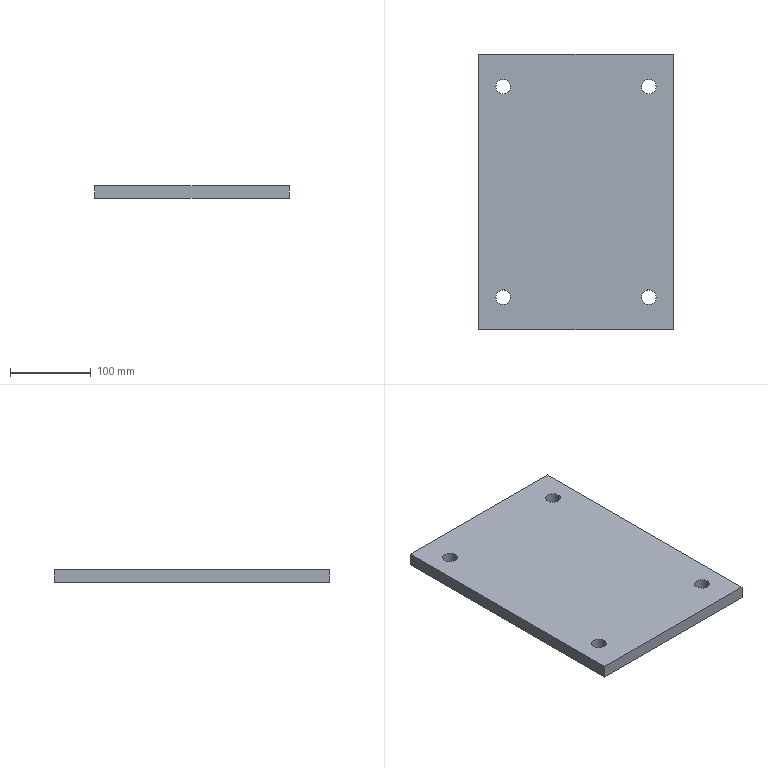Part | SolidWorks | features Extrusion 1 | 1 solid | 14 faces | box 240 x 340 x 16 mm | volume 1289314 mm3 | cylinder 8 | plane 6 | commonest cylinder face diameters 18 x8
STEP:
#1=CARTESIAN_POINT('',(-99.,-130.,16.));
#2=VERTEX_POINT('',#1);
#3=CARTESIAN_POINT('',(-81.,-130.,16.));
#4=VERTEX_POINT('',#3);
#5=CARTESIAN_POINT('',(-90.,-130.,16.));
#6=DIRECTION('',(0.,0.,1.));
#7=DIRECTION('',(1.,0.,0.));
#8=AXIS2_PLACEMENT_3D('',#5,#6,#7);
#9=CIRCLE('',#8,9.);
#10=EDGE_CURVE('',#2,#4,#9,.T.);
#11=ORIENTED_EDGE('',*,*,#10,.T.);
#12=CARTESIAN_POINT('',(-81.,-130.,0.));
#13=VERTEX_POINT('',#12);
#14=CARTESIAN_POINT('',(-81.,-130.,16.));
#15=DIRECTION('',(0.,0.,-1.));
#16=VECTOR('',#15,1000.);
#17=LINE('',#14,#16);
#18=EDGE_CURVE('',#4,#13,#17,.T.);
#19=ORIENTED_EDGE('',*,*,#18,.T.);
#20=CARTESIAN_POINT('',(-99.,-130.,0.));
#21=VERTEX_POINT('',#20);
#22=CARTESIAN_POINT('',(-90.,-130.,0.));
#23=DIRECTION('',(0.,0.,1.));
#24=DIRECTION('',(1.,0.,0.));
#25=AXIS2_PLACEMENT_3D('',#22,#23,#24);
#26=CIRCLE('',#25,9.);
#27=EDGE_CURVE('',#21,#13,#26,.T.);
#28=ORIENTED_EDGE('',*,*,#27,.F.);
#29=CARTESIAN_POINT('',(-99.,-130.,16.));
#30=DIRECTION('',(0.,0.,-1.));
#31=VECTOR('',#30,1000.);
#32=LINE('',#29,#31);
#33=EDGE_CURVE('',#2,#21,#32,.T.);
#34=ORIENTED_EDGE('',*,*,#33,.F.);
#35=EDGE_LOOP('',(#11,#19,#28,#34));
#36=FACE_OUTER_BOUND('',#35,.T.);
#37=CARTESIAN_POINT('',(-90.,-130.,16.));
#38=DIRECTION('',(0.,0.,-1.));
#39=DIRECTION('',(-1.,0.,0.));
#40=AXIS2_PLACEMENT_3D('',#37,#38,#39);
#41=CYLINDRICAL_SURFACE('',#40,9.);
#42=ADVANCED_FACE('',(#36),#41,.F.);
#43=CARTESIAN_POINT('',(81.,-130.,16.));
#44=VERTEX_POINT('',#43);
#45=CARTESIAN_POINT('',(99.,-130.,16.));
#46=VERTEX_POINT('',#45);
#47=CARTESIAN_POINT('',(90.,-130.,16.));
#48=DIRECTION('',(0.,0.,1.));
#49=DIRECTION('',(1.,0.,0.));
#50=AXIS2_PLACEMENT_3D('',#47,#48,#49);
#51=CIRCLE('',#50,9.);
#52=EDGE_CURVE('',#44,#46,#51,.T.);
#53=ORIENTED_EDGE('',*,*,#52,.T.);
#54=CARTESIAN_POINT('',(99.,-130.,0.));
#55=VERTEX_POINT('',#54);
#56=CARTESIAN_POINT('',(99.,-130.,16.));
#57=DIRECTION('',(0.,0.,-1.));
#58=VECTOR('',#57,1000.);
#59=LINE('',#56,#58);
#60=EDGE_CURVE('',#46,#55,#59,.T.);
#61=ORIENTED_EDGE('',*,*,#60,.T.);
#62=CARTESIAN_POINT('',(81.,-130.,0.));
#63=VERTEX_POINT('',#62);
#64=CARTESIAN_POINT('',(90.,-130.,0.));
#65=DIRECTION('',(0.,0.,1.));
#66=DIRECTION('',(1.,0.,0.));
#67=AXIS2_PLACEMENT_3D('',#64,#65,#66);
#68=CIRCLE('',#67,9.);
#69=EDGE_CURVE('',#63,#55,#68,.T.);
#70=ORIENTED_EDGE('',*,*,#69,.F.);
#71=CARTESIAN_POINT('',(81.,-130.,16.));
#72=DIRECTION('',(0.,0.,-1.));
#73=VECTOR('',#72,1000.);
#74=LINE('',#71,#73);
#75=EDGE_CURVE('',#44,#63,#74,.T.);
#76=ORIENTED_EDGE('',*,*,#75,.F.);
#77=EDGE_LOOP('',(#53,#61,#70,#76));
#78=FACE_OUTER_BOUND('',#77,.T.);
#79=CARTESIAN_POINT('',(90.,-130.,16.));
#80=DIRECTION('',(0.,0.,-1.));
#81=DIRECTION('',(-1.,0.,0.));
#82=AXIS2_PLACEMENT_3D('',#79,#80,#81);
#83=CYLINDRICAL_SURFACE('',#82,9.);
#84=ADVANCED_FACE('',(#78),#83,.F.);
#85=CARTESIAN_POINT('',(81.,130.,16.));
#86=VERTEX_POINT('',#85);
#87=CARTESIAN_POINT('',(99.,130.,16.));
#88=VERTEX_POINT('',#87);
#89=CARTESIAN_POINT('',(90.,130.,16.));
#90=DIRECTION('',(0.,0.,1.));
#91=DIRECTION('',(1.,0.,0.));
#92=AXIS2_PLACEMENT_3D('',#89,#90,#91);
#93=CIRCLE('',#92,9.);
#94=EDGE_CURVE('',#86,#88,#93,.T.);
#95=ORIENTED_EDGE('',*,*,#94,.T.);
#96=CARTESIAN_POINT('',(99.,130.,0.));
#97=VERTEX_POINT('',#96);
#98=CARTESIAN_POINT('',(99.,130.,16.));
#99=DIRECTION('',(0.,0.,-1.));
#100=VECTOR('',#99,1000.);
#101=LINE('',#98,#100);
#102=EDGE_CURVE('',#88,#97,#101,.T.);
#103=ORIENTED_EDGE('',*,*,#102,.T.);
#104=CARTESIAN_POINT('',(81.,130.,0.));
#105=VERTEX_POINT('',#104);
#106=CARTESIAN_POINT('',(90.,130.,0.));
#107=DIRECTION('',(0.,0.,1.));
#108=DIRECTION('',(1.,0.,0.));
#109=AXIS2_PLACEMENT_3D('',#106,#107,#108);
#110=CIRCLE('',#109,9.);
#111=EDGE_CURVE('',#105,#97,#110,.T.);
#112=ORIENTED_EDGE('',*,*,#111,.F.);
#113=CARTESIAN_POINT('',(81.,130.,16.));
#114=DIRECTION('',(0.,0.,-1.));
#115=VECTOR('',#114,1000.);
#116=LINE('',#113,#115);
#117=EDGE_CURVE('',#86,#105,#116,.T.);
#118=ORIENTED_EDGE('',*,*,#117,.F.);
#119=EDGE_LOOP('',(#95,#103,#112,#118));
#120=FACE_OUTER_BOUND('',#119,.T.);
#121=CARTESIAN_POINT('',(90.,130.,16.));
#122=DIRECTION('',(0.,0.,-1.));
#123=DIRECTION('',(-1.,0.,0.));
#124=AXIS2_PLACEMENT_3D('',#121,#122,#123);
#125=CYLINDRICAL_SURFACE('',#124,9.);
#126=ADVANCED_FACE('',(#120),#125,.F.);
#127=CARTESIAN_POINT('',(-99.,130.,16.));
#128=VERTEX_POINT('',#127);
#129=CARTESIAN_POINT('',(-81.,130.,16.));
#130=VERTEX_POINT('',#129);
#131=CARTESIAN_POINT('',(-90.,130.,16.));
#132=DIRECTION('',(0.,0.,1.));
#133=DIRECTION('',(1.,0.,0.));
#134=AXIS2_PLACEMENT_3D('',#131,#132,#133);
#135=CIRCLE('',#134,9.);
#136=EDGE_CURVE('',#128,#130,#135,.T.);
#137=ORIENTED_EDGE('',*,*,#136,.T.);
#138=CARTESIAN_POINT('',(-81.,130.,0.));
#139=VERTEX_POINT('',#138);
#140=CARTESIAN_POINT('',(-81.,130.,16.));
#141=DIRECTION('',(0.,0.,-1.));
#142=VECTOR('',#141,1000.);
#143=LINE('',#140,#142);
#144=EDGE_CURVE('',#130,#139,#143,.T.);
#145=ORIENTED_EDGE('',*,*,#144,.T.);
#146=CARTESIAN_POINT('',(-99.,130.,0.));
#147=VERTEX_POINT('',#146);
#148=CARTESIAN_POINT('',(-90.,130.,0.));
#149=DIRECTION('',(0.,0.,1.));
#150=DIRECTION('',(1.,0.,0.));
#151=AXIS2_PLACEMENT_3D('',#148,#149,#150);
#152=CIRCLE('',#151,9.);
#153=EDGE_CURVE('',#147,#139,#152,.T.);
#154=ORIENTED_EDGE('',*,*,#153,.F.);
#155=CARTESIAN_POINT('',(-99.,130.,16.));
#156=DIRECTION('',(0.,0.,-1.));
#157=VECTOR('',#156,1000.);
#158=LINE('',#155,#157);
#159=EDGE_CURVE('',#128,#147,#158,.T.);
#160=ORIENTED_EDGE('',*,*,#159,.F.);
#161=EDGE_LOOP('',(#137,#145,#154,#160));
#162=FACE_OUTER_BOUND('',#161,.T.);
#163=CARTESIAN_POINT('',(-90.,130.,16.));
#164=DIRECTION('',(0.,0.,-1.));
#165=DIRECTION('',(-1.,0.,0.));
#166=AXIS2_PLACEMENT_3D('',#163,#164,#165);
#167=CYLINDRICAL_SURFACE('',#166,9.);
#168=ADVANCED_FACE('',(#162),#167,.F.);
#169=CARTESIAN_POINT('',(120.,-170.,16.));
#170=VERTEX_POINT('',#169);
#171=CARTESIAN_POINT('',(120.,170.,16.));
#172=VERTEX_POINT('',#171);
#173=CARTESIAN_POINT('',(120.,-170.,16.));
#174=DIRECTION('',(0.,1.,0.));
#175=VECTOR('',#174,1000.);
#176=LINE('',#173,#175);
#177=EDGE_CURVE('',#170,#172,#176,.T.);
#178=ORIENTED_EDGE('',*,*,#177,.T.);
#179=CARTESIAN_POINT('',(-120.,170.,16.));
#180=VERTEX_POINT('',#179);
#181=CARTESIAN_POINT('',(-120.,170.,16.));
#182=DIRECTION('',(-1.,0.,0.));
#183=VECTOR('',#182,1000.);
#184=LINE('',#181,#183);
#185=EDGE_CURVE('',#172,#180,#184,.T.);
#186=ORIENTED_EDGE('',*,*,#185,.T.);
#187=CARTESIAN_POINT('',(-120.,-170.,16.));
#188=VERTEX_POINT('',#187);
#189=CARTESIAN_POINT('',(-120.,-170.,16.));
#190=DIRECTION('',(0.,-1.,0.));
#191=VECTOR('',#190,1000.);
#192=LINE('',#189,#191);
#193=EDGE_CURVE('',#180,#188,#192,.T.);
#194=ORIENTED_EDGE('',*,*,#193,.T.);
#195=CARTESIAN_POINT('',(-120.,-170.,16.));
#196=DIRECTION('',(1.,0.,0.));
#197=VECTOR('',#196,1000.);
#198=LINE('',#195,#197);
#199=EDGE_CURVE('',#188,#170,#198,.T.);
#200=ORIENTED_EDGE('',*,*,#199,.T.);
#201=EDGE_LOOP('',(#178,#186,#194,#200));
#202=FACE_OUTER_BOUND('',#201,.T.);
#203=ORIENTED_EDGE('',*,*,#136,.F.);
#204=CARTESIAN_POINT('',(-90.,130.,16.));
#205=DIRECTION('',(0.,0.,1.));
#206=DIRECTION('',(1.,0.,0.));
#207=AXIS2_PLACEMENT_3D('',#204,#205,#206);
#208=CIRCLE('',#207,9.);
#209=EDGE_CURVE('',#130,#128,#208,.T.);
#210=ORIENTED_EDGE('',*,*,#209,.F.);
#211=EDGE_LOOP('',(#203,#210));
#212=FACE_BOUND('',#211,.T.);
#213=ORIENTED_EDGE('',*,*,#94,.F.);
#214=CARTESIAN_POINT('',(90.,130.,16.));
#215=DIRECTION('',(0.,0.,1.));
#216=DIRECTION('',(1.,0.,0.));
#217=AXIS2_PLACEMENT_3D('',#214,#215,#216);
#218=CIRCLE('',#217,9.);
#219=EDGE_CURVE('',#88,#86,#218,.T.);
#220=ORIENTED_EDGE('',*,*,#219,.F.);
#221=EDGE_LOOP('',(#213,#220));
#222=FACE_BOUND('',#221,.T.);
#223=ORIENTED_EDGE('',*,*,#52,.F.);
#224=CARTESIAN_POINT('',(90.,-130.,16.));
#225=DIRECTION('',(0.,0.,1.));
#226=DIRECTION('',(1.,0.,0.));
#227=AXIS2_PLACEMENT_3D('',#224,#225,#226);
#228=CIRCLE('',#227,9.);
#229=EDGE_CURVE('',#46,#44,#228,.T.);
#230=ORIENTED_EDGE('',*,*,#229,.F.);
#231=EDGE_LOOP('',(#223,#230));
#232=FACE_BOUND('',#231,.T.);
#233=ORIENTED_EDGE('',*,*,#10,.F.);
#234=CARTESIAN_POINT('',(-90.,-130.,16.));
#235=DIRECTION('',(0.,0.,1.));
#236=DIRECTION('',(1.,0.,0.));
#237=AXIS2_PLACEMENT_3D('',#234,#235,#236);
#238=CIRCLE('',#237,9.);
#239=EDGE_CURVE('',#4,#2,#238,.T.);
#240=ORIENTED_EDGE('',*,*,#239,.F.);
#241=EDGE_LOOP('',(#233,#240));
#242=FACE_BOUND('',#241,.T.);
#243=CARTESIAN_POINT('',(0.,0.,16.));
#244=DIRECTION('',(0.,0.,-1.));
#245=DIRECTION('',(-1.,0.,0.));
#246=AXIS2_PLACEMENT_3D('',#243,#244,#245);
#247=PLANE('',#246);
#248=ADVANCED_FACE('',(#202,#212,#222,#232,#242),#247,.F.);
#249=ORIENTED_EDGE('',*,*,#69,.T.);
#250=CARTESIAN_POINT('',(90.,-130.,0.));
#251=DIRECTION('',(0.,0.,1.));
#252=DIRECTION('',(1.,0.,0.));
#253=AXIS2_PLACEMENT_3D('',#250,#251,#252);
#254=CIRCLE('',#253,9.);
#255=EDGE_CURVE('',#55,#63,#254,.T.);
#256=ORIENTED_EDGE('',*,*,#255,.T.);
#257=EDGE_LOOP('',(#249,#256));
#258=FACE_BOUND('',#257,.T.);
#259=ORIENTED_EDGE('',*,*,#153,.T.);
#260=CARTESIAN_POINT('',(-90.,130.,0.));
#261=DIRECTION('',(0.,0.,1.));
#262=DIRECTION('',(1.,0.,0.));
#263=AXIS2_PLACEMENT_3D('',#260,#261,#262);
#264=CIRCLE('',#263,9.);
#265=EDGE_CURVE('',#139,#147,#264,.T.);
#266=ORIENTED_EDGE('',*,*,#265,.T.);
#267=EDGE_LOOP('',(#259,#266));
#268=FACE_BOUND('',#267,.T.);
#269=CARTESIAN_POINT('',(120.,-170.,0.));
#270=VERTEX_POINT('',#269);
#271=CARTESIAN_POINT('',(120.,170.,0.));
#272=VERTEX_POINT('',#271);
#273=CARTESIAN_POINT('',(120.,-170.,0.));
#274=DIRECTION('',(0.,1.,0.));
#275=VECTOR('',#274,1000.);
#276=LINE('',#273,#275);
#277=EDGE_CURVE('',#270,#272,#276,.T.);
#278=ORIENTED_EDGE('',*,*,#277,.F.);
#279=CARTESIAN_POINT('',(-120.,-170.,0.));
#280=VERTEX_POINT('',#279);
#281=CARTESIAN_POINT('',(-120.,-170.,0.));
#282=DIRECTION('',(1.,0.,0.));
#283=VECTOR('',#282,1000.);
#284=LINE('',#281,#283);
#285=EDGE_CURVE('',#280,#270,#284,.T.);
#286=ORIENTED_EDGE('',*,*,#285,.F.);
#287=CARTESIAN_POINT('',(-120.,170.,0.));
#288=VERTEX_POINT('',#287);
#289=CARTESIAN_POINT('',(-120.,-170.,0.));
#290=DIRECTION('',(0.,-1.,0.));
#291=VECTOR('',#290,1000.);
#292=LINE('',#289,#291);
#293=EDGE_CURVE('',#288,#280,#292,.T.);
#294=ORIENTED_EDGE('',*,*,#293,.F.);
#295=CARTESIAN_POINT('',(-120.,170.,0.));
#296=DIRECTION('',(-1.,0.,0.));
#297=VECTOR('',#296,1000.);
#298=LINE('',#295,#297);
#299=EDGE_CURVE('',#272,#288,#298,.T.);
#300=ORIENTED_EDGE('',*,*,#299,.F.);
#301=EDGE_LOOP('',(#278,#286,#294,#300));
#302=FACE_OUTER_BOUND('',#301,.T.);
#303=ORIENTED_EDGE('',*,*,#111,.T.);
#304=CARTESIAN_POINT('',(90.,130.,0.));
#305=DIRECTION('',(0.,0.,1.));
#306=DIRECTION('',(1.,0.,0.));
#307=AXIS2_PLACEMENT_3D('',#304,#305,#306);
#308=CIRCLE('',#307,9.);
#309=EDGE_CURVE('',#97,#105,#308,.T.);
#310=ORIENTED_EDGE('',*,*,#309,.T.);
#311=EDGE_LOOP('',(#303,#310));
#312=FACE_BOUND('',#311,.T.);
#313=ORIENTED_EDGE('',*,*,#27,.T.);
#314=CARTESIAN_POINT('',(-90.,-130.,0.));
#315=DIRECTION('',(0.,0.,1.));
#316=DIRECTION('',(1.,0.,0.));
#317=AXIS2_PLACEMENT_3D('',#314,#315,#316);
#318=CIRCLE('',#317,9.);
#319=EDGE_CURVE('',#13,#21,#318,.T.);
#320=ORIENTED_EDGE('',*,*,#319,.T.);
#321=EDGE_LOOP('',(#313,#320));
#322=FACE_BOUND('',#321,.T.);
#323=CARTESIAN_POINT('',(0.,0.,0.));
#324=DIRECTION('',(0.,0.,-1.));
#325=DIRECTION('',(-1.,0.,0.));
#326=AXIS2_PLACEMENT_3D('',#323,#324,#325);
#327=PLANE('',#326);
#328=ADVANCED_FACE('',(#258,#268,#302,#312,#322),#327,.T.);
#329=ORIENTED_EDGE('',*,*,#277,.T.);
#330=CARTESIAN_POINT('',(120.,170.,16.));
#331=DIRECTION('',(0.,0.,-1.));
#332=VECTOR('',#331,1000.);
#333=LINE('',#330,#332);
#334=EDGE_CURVE('',#172,#272,#333,.T.);
#335=ORIENTED_EDGE('',*,*,#334,.F.);
#336=ORIENTED_EDGE('',*,*,#177,.F.);
#337=CARTESIAN_POINT('',(120.,-170.,16.));
#338=DIRECTION('',(0.,0.,-1.));
#339=VECTOR('',#338,1000.);
#340=LINE('',#337,#339);
#341=EDGE_CURVE('',#170,#270,#340,.T.);
#342=ORIENTED_EDGE('',*,*,#341,.T.);
#343=EDGE_LOOP('',(#329,#335,#336,#342));
#344=FACE_OUTER_BOUND('',#343,.T.);
#345=CARTESIAN_POINT('',(120.,-170.,16.));
#346=DIRECTION('',(-1.,0.,0.));
#347=DIRECTION('',(0.,0.,1.));
#348=AXIS2_PLACEMENT_3D('',#345,#346,#347);
#349=PLANE('',#348);
#350=ADVANCED_FACE('',(#344),#349,.F.);
#351=ORIENTED_EDGE('',*,*,#299,.T.);
#352=CARTESIAN_POINT('',(-120.,170.,16.));
#353=DIRECTION('',(0.,0.,-1.));
#354=VECTOR('',#353,1000.);
#355=LINE('',#352,#354);
#356=EDGE_CURVE('',#180,#288,#355,.T.);
#357=ORIENTED_EDGE('',*,*,#356,.F.);
#358=ORIENTED_EDGE('',*,*,#185,.F.);
#359=ORIENTED_EDGE('',*,*,#334,.T.);
#360=EDGE_LOOP('',(#351,#357,#358,#359));
#361=FACE_OUTER_BOUND('',#360,.T.);
#362=CARTESIAN_POINT('',(-120.,170.,16.));
#363=DIRECTION('',(0.,-1.,0.));
#364=DIRECTION('',(0.,0.,-1.));
#365=AXIS2_PLACEMENT_3D('',#362,#363,#364);
#366=PLANE('',#365);
#367=ADVANCED_FACE('',(#361),#366,.F.);
#368=ORIENTED_EDGE('',*,*,#293,.T.);
#369=CARTESIAN_POINT('',(-120.,-170.,16.));
#370=DIRECTION('',(0.,0.,-1.));
#371=VECTOR('',#370,1000.);
#372=LINE('',#369,#371);
#373=EDGE_CURVE('',#188,#280,#372,.T.);
#374=ORIENTED_EDGE('',*,*,#373,.F.);
#375=ORIENTED_EDGE('',*,*,#193,.F.);
#376=ORIENTED_EDGE('',*,*,#356,.T.);
#377=EDGE_LOOP('',(#368,#374,#375,#376));
#378=FACE_OUTER_BOUND('',#377,.T.);
#379=CARTESIAN_POINT('',(-120.,-170.,16.));
#380=DIRECTION('',(1.,0.,0.));
#381=DIRECTION('',(0.,0.,-1.));
#382=AXIS2_PLACEMENT_3D('',#379,#380,#381);
#383=PLANE('',#382);
#384=ADVANCED_FACE('',(#378),#383,.F.);
#385=ORIENTED_EDGE('',*,*,#285,.T.);
#386=ORIENTED_EDGE('',*,*,#341,.F.);
#387=ORIENTED_EDGE('',*,*,#199,.F.);
#388=ORIENTED_EDGE('',*,*,#373,.T.);
#389=EDGE_LOOP('',(#385,#386,#387,#388));
#390=FACE_OUTER_BOUND('',#389,.T.);
#391=CARTESIAN_POINT('',(-120.,-170.,16.));
#392=DIRECTION('',(0.,1.,0.));
#393=DIRECTION('',(0.,0.,1.));
#394=AXIS2_PLACEMENT_3D('',#391,#392,#393);
#395=PLANE('',#394);
#396=ADVANCED_FACE('',(#390),#395,.F.);
#397=ORIENTED_EDGE('',*,*,#144,.F.);
#398=ORIENTED_EDGE('',*,*,#209,.T.);
#399=ORIENTED_EDGE('',*,*,#159,.T.);
#400=ORIENTED_EDGE('',*,*,#265,.F.);
#401=EDGE_LOOP('',(#397,#398,#399,#400));
#402=FACE_OUTER_BOUND('',#401,.T.);
#403=CARTESIAN_POINT('',(-90.,130.,16.));
#404=DIRECTION('',(0.,0.,-1.));
#405=DIRECTION('',(-1.,0.,0.));
#406=AXIS2_PLACEMENT_3D('',#403,#404,#405);
#407=CYLINDRICAL_SURFACE('',#406,9.);
#408=ADVANCED_FACE('',(#402),#407,.F.);
#409=ORIENTED_EDGE('',*,*,#102,.F.);
#410=ORIENTED_EDGE('',*,*,#219,.T.);
#411=ORIENTED_EDGE('',*,*,#117,.T.);
#412=ORIENTED_EDGE('',*,*,#309,.F.);
#413=EDGE_LOOP('',(#409,#410,#411,#412));
#414=FACE_OUTER_BOUND('',#413,.T.);
#415=CARTESIAN_POINT('',(90.,130.,16.));
#416=DIRECTION('',(0.,0.,-1.));
#417=DIRECTION('',(-1.,0.,0.));
#418=AXIS2_PLACEMENT_3D('',#415,#416,#417);
#419=CYLINDRICAL_SURFACE('',#418,9.);
#420=ADVANCED_FACE('',(#414),#419,.F.);
#421=ORIENTED_EDGE('',*,*,#60,.F.);
#422=ORIENTED_EDGE('',*,*,#229,.T.);
#423=ORIENTED_EDGE('',*,*,#75,.T.);
#424=ORIENTED_EDGE('',*,*,#255,.F.);
#425=EDGE_LOOP('',(#421,#422,#423,#424));
#426=FACE_OUTER_BOUND('',#425,.T.);
#427=CARTESIAN_POINT('',(90.,-130.,16.));
#428=DIRECTION('',(0.,0.,-1.));
#429=DIRECTION('',(-1.,0.,0.));
#430=AXIS2_PLACEMENT_3D('',#427,#428,#429);
#431=CYLINDRICAL_SURFACE('',#430,9.);
#432=ADVANCED_FACE('',(#426),#431,.F.);
#433=ORIENTED_EDGE('',*,*,#18,.F.);
#434=ORIENTED_EDGE('',*,*,#239,.T.);
#435=ORIENTED_EDGE('',*,*,#33,.T.);
#436=ORIENTED_EDGE('',*,*,#319,.F.);
#437=EDGE_LOOP('',(#433,#434,#435,#436));
#438=FACE_OUTER_BOUND('',#437,.T.);
#439=CARTESIAN_POINT('',(-90.,-130.,16.));
#440=DIRECTION('',(0.,0.,-1.));
#441=DIRECTION('',(-1.,0.,0.));
#442=AXIS2_PLACEMENT_3D('',#439,#440,#441);
#443=CYLINDRICAL_SURFACE('',#442,9.);
#444=ADVANCED_FACE('',(#438),#443,.F.);
#445=CLOSED_SHELL('',(#42,#84,#126,#168,#248,#328,#350,#367,#384,#396,#408,#420,#432,#444));
#446=MANIFOLD_SOLID_BREP('',#445);
#447=CARTESIAN_POINT('',(0.,0.,0.));
#448=DIRECTION('',(0.,0.,1.));
#449=DIRECTION('',(1.,0.,0.));
#450=AXIS2_PLACEMENT_3D('',#447,#448,#449);
#451=(LENGTH_UNIT()NAMED_UNIT(*)SI_UNIT(.MILLI.,.METRE.));
#452=UNCERTAINTY_MEASURE_WITH_UNIT(LENGTH_MEASURE(0.00001),#451,'','');
#453=(NAMED_UNIT(*)PLANE_ANGLE_UNIT()SI_UNIT($,.RADIAN.));
#454=(NAMED_UNIT(*)SI_UNIT($,.STERADIAN.)SOLID_ANGLE_UNIT());
#455=(GEOMETRIC_REPRESENTATION_CONTEXT(3)GLOBAL_UNCERTAINTY_ASSIGNED_CONTEXT((#452))GLOBAL_UNIT_ASSIGNED_CONTEXT((#451,#453,#454))REPRESENTATION_CONTEXT('',''));
#456=ADVANCED_BREP_SHAPE_REPRESENTATION('',(#446,#450),#455);